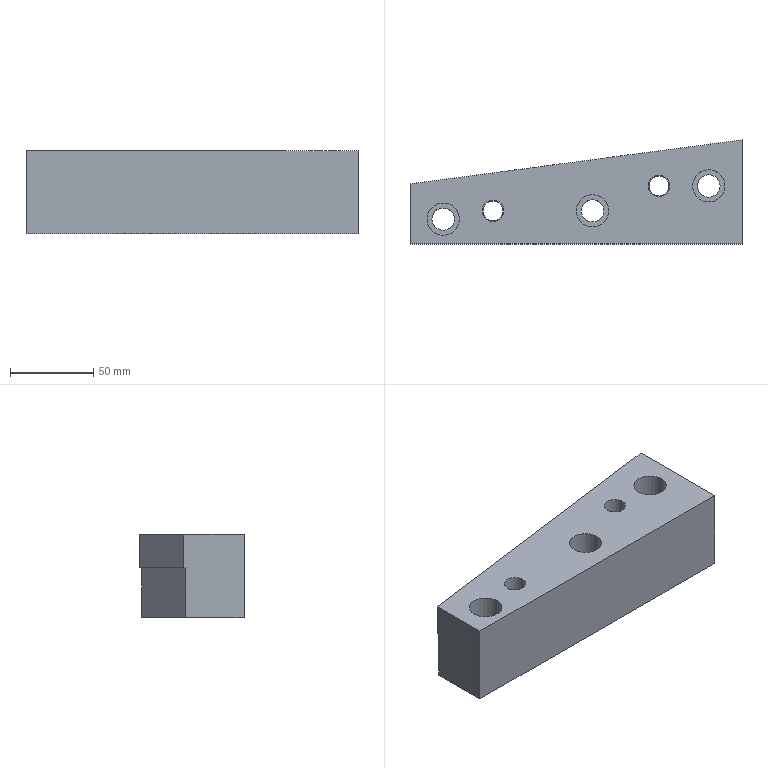Part | NX | features solid 2 | 1 solid | 23 faces | box 200 x 62.717 x 50 mm | volume 447168 mm3 | plane 11 | cylinder 10 | spline 2 | commonest cylinder face diameters 13.5 x3 19.5 x3 12 x2 13 x2
STEP:
#1=CARTESIAN_POINT('',(251.,105.,-50.));
#2=VERTEX_POINT('',#1);
#3=CARTESIAN_POINT('',(245.,105.,-50.));
#4=DIRECTION('',(0.,0.,1.));
#5=DIRECTION('',(1.,0.,0.));
#6=AXIS2_PLACEMENT_3D('',#3,#4,#5);
#7=CIRCLE('',#6,6.);
#8=EDGE_CURVE('',#2,#2,#7,.T.);
#9=ORIENTED_EDGE('',*,*,#8,.T.);
#10=EDGE_LOOP('',(#9));
#11=FACE_BOUND('',#10,.T.);
#12=CARTESIAN_POINT('',(151.,90.,-50.));
#13=VERTEX_POINT('',#12);
#14=CARTESIAN_POINT('',(145.,90.,-50.));
#15=DIRECTION('',(0.,0.,1.));
#16=DIRECTION('',(1.,0.,0.));
#17=AXIS2_PLACEMENT_3D('',#14,#15,#16);
#18=CIRCLE('',#17,6.);
#19=EDGE_CURVE('',#13,#13,#18,.T.);
#20=ORIENTED_EDGE('',*,*,#19,.T.);
#21=EDGE_LOOP('',(#20));
#22=FACE_BOUND('',#21,.T.);
#23=CARTESIAN_POINT('',(211.75,90.,-50.));
#24=VERTEX_POINT('',#23);
#25=CARTESIAN_POINT('',(205.,90.,-50.));
#26=DIRECTION('',(0.,0.,1.));
#27=DIRECTION('',(1.,0.,0.));
#28=AXIS2_PLACEMENT_3D('',#25,#26,#27);
#29=CIRCLE('',#28,6.75);
#30=EDGE_CURVE('',#24,#24,#29,.T.);
#31=ORIENTED_EDGE('',*,*,#30,.T.);
#32=EDGE_LOOP('',(#31));
#33=FACE_BOUND('',#32,.T.);
#34=CARTESIAN_POINT('',(281.75,105.,-50.));
#35=VERTEX_POINT('',#34);
#36=CARTESIAN_POINT('',(275.,105.,-50.));
#37=DIRECTION('',(0.,0.,1.));
#38=DIRECTION('',(1.,0.,0.));
#39=AXIS2_PLACEMENT_3D('',#36,#37,#38);
#40=CIRCLE('',#39,6.75);
#41=EDGE_CURVE('',#35,#35,#40,.T.);
#42=ORIENTED_EDGE('',*,*,#41,.T.);
#43=EDGE_LOOP('',(#42));
#44=FACE_BOUND('',#43,.T.);
#45=CARTESIAN_POINT('',(121.75,85.,-50.));
#46=VERTEX_POINT('',#45);
#47=CARTESIAN_POINT('',(115.,85.,-50.));
#48=DIRECTION('',(0.,0.,1.));
#49=DIRECTION('',(1.,0.,0.));
#50=AXIS2_PLACEMENT_3D('',#47,#48,#49);
#51=CIRCLE('',#50,6.75);
#52=EDGE_CURVE('',#46,#46,#51,.T.);
#53=ORIENTED_EDGE('',*,*,#52,.T.);
#54=EDGE_LOOP('',(#53));
#55=FACE_BOUND('',#54,.T.);
#56=CARTESIAN_POINT('',(95.,70.,-50.));
#57=VERTEX_POINT('',#56);
#58=CARTESIAN_POINT('',(95.,105.2,-50.));
#59=VERTEX_POINT('',#58);
#60=CARTESIAN_POINT('',(95.,35.09,-50.));
#61=DIRECTION('',(0.,1.,0.));
#62=VECTOR('',#61,1000.);
#63=LINE('',#60,#62);
#64=EDGE_CURVE('',#57,#59,#63,.T.);
#65=ORIENTED_EDGE('',*,*,#64,.T.);
#66=CARTESIAN_POINT('',(295.,131.707,-50.));
#67=VERTEX_POINT('',#66);
#68=CARTESIAN_POINT('',(95.,105.2,-50.));
#69=CARTESIAN_POINT('',(128.341,109.558,-50.));
#70=CARTESIAN_POINT('',(178.34,116.191,-50.));
#71=CARTESIAN_POINT('',(245.019,124.939,-50.));
#72=CARTESIAN_POINT('',(278.357,129.318,-50.));
#73=CARTESIAN_POINT('',(295.,131.707,-50.));
#74=B_SPLINE_CURVE_WITH_KNOTS('',3,(#68,#69,#70,#71,#72,#73),.UNSPECIFIED.,.F.,.F.,(4,1,1,4),(0.,0.1009,0.1513,0.2017),.UNSPECIFIED.);
#75=EDGE_CURVE('',#59,#67,#74,.T.);
#76=ORIENTED_EDGE('',*,*,#75,.T.);
#77=CARTESIAN_POINT('',(295.,70.,-50.));
#78=VERTEX_POINT('',#77);
#79=CARTESIAN_POINT('',(295.,35.09,-50.));
#80=DIRECTION('',(0.,-1.,0.));
#81=VECTOR('',#80,1000.);
#82=LINE('',#79,#81);
#83=EDGE_CURVE('',#67,#78,#82,.T.);
#84=ORIENTED_EDGE('',*,*,#83,.T.);
#85=CARTESIAN_POINT('',(-415.478,70.,-50.));
#86=DIRECTION('',(-1.,0.,0.));
#87=VECTOR('',#86,1000.);
#88=LINE('',#85,#87);
#89=EDGE_CURVE('',#78,#57,#88,.T.);
#90=ORIENTED_EDGE('',*,*,#89,.T.);
#91=EDGE_LOOP('',(#65,#76,#84,#90));
#92=FACE_BOUND('',#91,.T.);
#93=CARTESIAN_POINT('',(-415.478,35.09,-50.));
#94=DIRECTION('',(0.,0.,1.));
#95=DIRECTION('',(1.,0.,0.));
#96=AXIS2_PLACEMENT_3D('',#93,#94,#95);
#97=PLANE('',#96);
#98=ADVANCED_FACE('',(#11,#22,#33,#44,#55,#92),#97,.F.);
#99=CARTESIAN_POINT('',(295.,70.,0.));
#100=VERTEX_POINT('',#99);
#101=CARTESIAN_POINT('',(295.,70.,0.));
#102=DIRECTION('',(0.,0.,1.));
#103=VECTOR('',#102,1000.);
#104=LINE('',#101,#103);
#105=EDGE_CURVE('',#78,#100,#104,.T.);
#106=ORIENTED_EDGE('',*,*,#105,.T.);
#107=CARTESIAN_POINT('',(95.,70.,0.));
#108=VERTEX_POINT('',#107);
#109=CARTESIAN_POINT('',(-470.381,70.,0.));
#110=DIRECTION('',(1.,0.,0.));
#111=VECTOR('',#110,1000.);
#112=LINE('',#109,#111);
#113=EDGE_CURVE('',#108,#100,#112,.T.);
#114=ORIENTED_EDGE('',*,*,#113,.F.);
#115=CARTESIAN_POINT('',(95.,70.,0.));
#116=DIRECTION('',(0.,0.,-1.));
#117=VECTOR('',#116,1000.);
#118=LINE('',#115,#117);
#119=EDGE_CURVE('',#108,#57,#118,.T.);
#120=ORIENTED_EDGE('',*,*,#119,.T.);
#121=ORIENTED_EDGE('',*,*,#89,.F.);
#122=EDGE_LOOP('',(#106,#114,#120,#121));
#123=FACE_BOUND('',#122,.T.);
#124=CARTESIAN_POINT('',(180.,70.,0.));
#125=DIRECTION('',(0.,1.,0.));
#126=DIRECTION('',(0.,0.,1.));
#127=AXIS2_PLACEMENT_3D('',#124,#125,#126);
#128=PLANE('',#127);
#129=ADVANCED_FACE('',(#123),#128,.F.);
#130=CARTESIAN_POINT('',(238.5,105.,0.));
#131=VERTEX_POINT('',#130);
#132=CARTESIAN_POINT('',(245.,105.,0.));
#133=DIRECTION('',(0.,0.,-1.));
#134=DIRECTION('',(-1.,0.,0.));
#135=AXIS2_PLACEMENT_3D('',#132,#133,#134);
#136=CIRCLE('',#135,6.5);
#137=EDGE_CURVE('',#131,#131,#136,.T.);
#138=ORIENTED_EDGE('',*,*,#137,.T.);
#139=EDGE_LOOP('',(#138));
#140=FACE_BOUND('',#139,.T.);
#141=CARTESIAN_POINT('',(138.5,90.,0.));
#142=VERTEX_POINT('',#141);
#143=CARTESIAN_POINT('',(145.,90.,0.));
#144=DIRECTION('',(0.,0.,-1.));
#145=DIRECTION('',(-1.,0.,0.));
#146=AXIS2_PLACEMENT_3D('',#143,#144,#145);
#147=CIRCLE('',#146,6.5);
#148=EDGE_CURVE('',#142,#142,#147,.T.);
#149=ORIENTED_EDGE('',*,*,#148,.T.);
#150=EDGE_LOOP('',(#149));
#151=FACE_BOUND('',#150,.T.);
#152=CARTESIAN_POINT('',(195.25,90.,0.));
#153=VERTEX_POINT('',#152);
#154=CARTESIAN_POINT('',(205.,90.,0.));
#155=DIRECTION('',(0.,0.,-1.));
#156=DIRECTION('',(-1.,0.,0.));
#157=AXIS2_PLACEMENT_3D('',#154,#155,#156);
#158=CIRCLE('',#157,9.75);
#159=EDGE_CURVE('',#153,#153,#158,.T.);
#160=ORIENTED_EDGE('',*,*,#159,.T.);
#161=EDGE_LOOP('',(#160));
#162=FACE_BOUND('',#161,.T.);
#163=CARTESIAN_POINT('',(265.25,105.,0.));
#164=VERTEX_POINT('',#163);
#165=CARTESIAN_POINT('',(275.,105.,0.));
#166=DIRECTION('',(0.,0.,-1.));
#167=DIRECTION('',(-1.,0.,0.));
#168=AXIS2_PLACEMENT_3D('',#165,#166,#167);
#169=CIRCLE('',#168,9.75);
#170=EDGE_CURVE('',#164,#164,#169,.T.);
#171=ORIENTED_EDGE('',*,*,#170,.T.);
#172=EDGE_LOOP('',(#171));
#173=FACE_BOUND('',#172,.T.);
#174=CARTESIAN_POINT('',(105.25,85.,0.));
#175=VERTEX_POINT('',#174);
#176=CARTESIAN_POINT('',(115.,85.,0.));
#177=DIRECTION('',(0.,0.,-1.));
#178=DIRECTION('',(-1.,0.,0.));
#179=AXIS2_PLACEMENT_3D('',#176,#177,#178);
#180=CIRCLE('',#179,9.75);
#181=EDGE_CURVE('',#175,#175,#180,.T.);
#182=ORIENTED_EDGE('',*,*,#181,.T.);
#183=EDGE_LOOP('',(#182));
#184=FACE_BOUND('',#183,.T.);
#185=CARTESIAN_POINT('',(295.,132.717,0.));
#186=VERTEX_POINT('',#185);
#187=CARTESIAN_POINT('',(295.,-222.,0.));
#188=DIRECTION('',(0.,1.,0.));
#189=VECTOR('',#188,1000.);
#190=LINE('',#187,#189);
#191=EDGE_CURVE('',#100,#186,#190,.T.);
#192=ORIENTED_EDGE('',*,*,#191,.T.);
#193=CARTESIAN_POINT('',(95.,106.209,0.));
#194=VERTEX_POINT('',#193);
#195=CARTESIAN_POINT('',(95.,106.209,0.));
#196=CARTESIAN_POINT('',(128.341,110.566,0.));
#197=CARTESIAN_POINT('',(178.341,117.199,0.));
#198=CARTESIAN_POINT('',(245.019,125.948,0.));
#199=CARTESIAN_POINT('',(278.357,130.326,0.));
#200=CARTESIAN_POINT('',(295.,132.717,0.));
#201=B_SPLINE_CURVE_WITH_KNOTS('',3,(#195,#196,#197,#198,#199,#200),.UNSPECIFIED.,.F.,.F.,(4,1,1,4),(0.,0.1009,0.1513,0.2017),.UNSPECIFIED.);
#202=EDGE_CURVE('',#194,#186,#201,.T.);
#203=ORIENTED_EDGE('',*,*,#202,.F.);
#204=CARTESIAN_POINT('',(95.,-222.,0.));
#205=DIRECTION('',(0.,-1.,0.));
#206=VECTOR('',#205,1000.);
#207=LINE('',#204,#206);
#208=EDGE_CURVE('',#194,#108,#207,.T.);
#209=ORIENTED_EDGE('',*,*,#208,.T.);
#210=ORIENTED_EDGE('',*,*,#113,.T.);
#211=EDGE_LOOP('',(#192,#203,#209,#210));
#212=FACE_BOUND('',#211,.T.);
#213=CARTESIAN_POINT('',(-470.381,-222.,0.));
#214=DIRECTION('',(0.,0.,-1.));
#215=DIRECTION('',(-1.,0.,0.));
#216=AXIS2_PLACEMENT_3D('',#213,#214,#215);
#217=PLANE('',#216);
#218=ADVANCED_FACE('',(#140,#151,#162,#173,#184,#212),#217,.F.);
#219=CARTESIAN_POINT('',(295.,132.717,-20.));
#220=VERTEX_POINT('',#219);
#221=CARTESIAN_POINT('',(295.,132.717,-10.));
#222=DIRECTION('',(0.,0.,-1.));
#223=VECTOR('',#222,1000.);
#224=LINE('',#221,#223);
#225=EDGE_CURVE('',#186,#220,#224,.T.);
#226=ORIENTED_EDGE('',*,*,#225,.T.);
#227=CARTESIAN_POINT('',(95.,106.209,-20.));
#228=VERTEX_POINT('',#227);
#229=CARTESIAN_POINT('',(-190.231,-121.49,-20.));
#230=CARTESIAN_POINT('',(-188.654,-121.152,-20.));
#231=CARTESIAN_POINT('',(-185.47,-120.627,-20.));
#232=CARTESIAN_POINT('',(-180.656,-120.141,-20.));
#233=CARTESIAN_POINT('',(-175.882,-119.326,-20.));
#234=CARTESIAN_POINT('',(-169.679,-117.528,-20.));
#235=CARTESIAN_POINT('',(-162.185,-114.539,-20.));
#236=CARTESIAN_POINT('',(-153.086,-111.254,-20.));
#237=CARTESIAN_POINT('',(-144.031,-107.845,-20.));
#238=CARTESIAN_POINT('',(-136.465,-105.061,-20.));
#239=CARTESIAN_POINT('',(-130.418,-102.814,-20.));
#240=CARTESIAN_POINT('',(-125.812,-101.329,-20.));
#241=CARTESIAN_POINT('',(-121.306,-99.566,-20.));
#242=CARTESIAN_POINT('',(-116.876,-97.626,-20.));
#243=CARTESIAN_POINT('',(-112.335,-95.923,-20.));
#244=CARTESIAN_POINT('',(-107.564,-95.05,-20.));
#245=CARTESIAN_POINT('',(-102.756,-94.525,-20.));
#246=CARTESIAN_POINT('',(-96.349,-93.771,-20.));
#247=CARTESIAN_POINT('',(-89.902,-93.468,-20.));
#248=CARTESIAN_POINT('',(-83.452,-93.448,-20.));
#249=CARTESIAN_POINT('',(-77.002,-93.469,-20.));
#250=CARTESIAN_POINT('',(-68.939,-93.411,-20.));
#251=CARTESIAN_POINT('',(-56.04,-93.3,-20.));
#252=CARTESIAN_POINT('',(-33.465,-93.184,-20.));
#253=CARTESIAN_POINT('',(-7.666,-93.074,-20.));
#254=CARTESIAN_POINT('',(14.907,-92.653,-20.));
#255=CARTESIAN_POINT('',(27.794,-92.068,-20.));
#256=CARTESIAN_POINT('',(40.668,-91.245,-20.));
#257=CARTESIAN_POINT('',(51.917,-90.291,-20.));
#258=CARTESIAN_POINT('',(61.528,-89.174,-20.));
#259=CARTESIAN_POINT('',(67.939,-88.466,-20.));
#260=CARTESIAN_POINT('',(79.125,-86.95,-20.));
#261=CARTESIAN_POINT('',(95.161,-85.253,-20.));
#262=CARTESIAN_POINT('',(114.404,-83.21,-20.));
#263=CARTESIAN_POINT('',(133.568,-80.524,-20.));
#264=CARTESIAN_POINT('',(152.734,-77.861,-20.));
#265=CARTESIAN_POINT('',(171.916,-75.326,-20.));
#266=CARTESIAN_POINT('',(191.055,-72.413,-20.));
#267=CARTESIAN_POINT('',(207.17,-71.468,-20.));
#268=CARTESIAN_POINT('',(219.951,-69.697,-20.));
#269=CARTESIAN_POINT('',(232.724,-67.899,-20.));
#270=CARTESIAN_POINT('',(248.708,-65.766,-20.));
#271=CARTESIAN_POINT('',(267.87,-63.074,-20.));
#272=CARTESIAN_POINT('',(287.038,-60.44,-20.));
#273=CARTESIAN_POINT('',(301.448,-58.682,-20.));
#274=CARTESIAN_POINT('',(310.976,-56.987,-20.));
#275=CARTESIAN_POINT('',(314.916,-56.135,-20.));
#276=CARTESIAN_POINT('',(318.052,-55.382,-20.));
#277=CARTESIAN_POINT('',(320.39,-54.76,-20.));
#278=CARTESIAN_POINT('',(322.686,-53.981,-20.));
#279=CARTESIAN_POINT('',(325.595,-52.578,-20.));
#280=CARTESIAN_POINT('',(328.769,-50.098,-20.));
#281=CARTESIAN_POINT('',(332.247,-46.69,-20.));
#282=CARTESIAN_POINT('',(335.795,-43.406,-20.));
#283=CARTESIAN_POINT('',(343.661,-37.758,-20.));
#284=CARTESIAN_POINT('',(355.164,-28.914,-20.));
#285=CARTESIAN_POINT('',(370.422,-17.018,-20.));
#286=CARTESIAN_POINT('',(383.264,-7.249,-20.));
#287=CARTESIAN_POINT('',(392.416,-0.6713,-20.));
#288=CARTESIAN_POINT('',(396.953,2.733,-20.));
#289=CARTESIAN_POINT('',(398.886,5.372,-20.));
#290=CARTESIAN_POINT('',(399.725,7.654,-20.));
#291=CARTESIAN_POINT('',(399.76,10.078,-20.));
#292=CARTESIAN_POINT('',(399.483,13.317,-20.));
#293=CARTESIAN_POINT('',(399.712,17.34,-20.));
#294=CARTESIAN_POINT('',(399.612,22.179,-20.));
#295=CARTESIAN_POINT('',(399.633,31.854,-20.));
#296=CARTESIAN_POINT('',(399.593,46.366,-20.));
#297=CARTESIAN_POINT('',(399.637,62.491,-20.));
#298=CARTESIAN_POINT('',(399.588,73.779,-20.));
#299=CARTESIAN_POINT('',(399.652,79.422,-20.));
#300=CARTESIAN_POINT('',(399.59,82.647,-20.));
#301=CARTESIAN_POINT('',(399.564,85.065,-20.));
#302=CARTESIAN_POINT('',(399.725,87.486,-20.));
#303=CARTESIAN_POINT('',(399.756,89.902,-20.));
#304=CARTESIAN_POINT('',(399.247,92.301,-20.));
#305=CARTESIAN_POINT('',(397.362,95.008,-20.));
#306=CARTESIAN_POINT('',(393.635,96.774,-20.));
#307=CARTESIAN_POINT('',(389.279,98.826,-20.));
#308=CARTESIAN_POINT('',(384.732,100.498,-20.));
#309=CARTESIAN_POINT('',(378.765,102.95,-20.));
#310=CARTESIAN_POINT('',(362.589,110.229,-20.));
#311=CARTESIAN_POINT('',(344.928,118.135,-20.));
#312=CARTESIAN_POINT('',(327.281,126.072,-20.));
#313=CARTESIAN_POINT('',(319.932,129.381,-20.));
#314=CARTESIAN_POINT('',(314.075,132.102,-20.));
#315=CARTESIAN_POINT('',(309.387,133.376,-20.));
#316=CARTESIAN_POINT('',(304.547,133.785,-20.));
#317=CARTESIAN_POINT('',(299.716,133.401,-20.));
#318=CARTESIAN_POINT('',(294.929,132.704,-20.));
#319=CARTESIAN_POINT('',(288.543,131.8,-20.));
#320=CARTESIAN_POINT('',(277.364,130.241,-20.));
#321=CARTESIAN_POINT('',(242.2,125.552,-20.));
#322=CARTESIAN_POINT('',(184.637,118.048,-20.));
#323=CARTESIAN_POINT('',(120.701,109.541,-20.));
#324=CARTESIAN_POINT('',(69.531,102.902,-20.));
#325=CARTESIAN_POINT('',(40.777,98.94,-20.));
#326=CARTESIAN_POINT('',(21.566,96.615,-20.));
#327=CARTESIAN_POINT('',(8.743,95.212,-20.));
#328=CARTESIAN_POINT('',(-7.301,93.575,-20.));
#329=CARTESIAN_POINT('',(-26.625,92.505,-20.));
#330=CARTESIAN_POINT('',(-45.971,92.017,-20.));
#331=CARTESIAN_POINT('',(-62.09,91.675,-20.));
#332=CARTESIAN_POINT('',(-74.987,91.256,-20.));
#333=CARTESIAN_POINT('',(-84.664,91.165,-20.));
#334=CARTESIAN_POINT('',(-94.319,91.781,-20.));
#335=CARTESIAN_POINT('',(-103.929,92.966,-20.));
#336=CARTESIAN_POINT('',(-113.495,94.403,-20.));
#337=CARTESIAN_POINT('',(-119.856,95.492,-20.));
#338=CARTESIAN_POINT('',(-122.997,96.222,-20.));
#339=B_SPLINE_CURVE_WITH_KNOTS('',3,(#229,#230,#231,#232,#233,#234,#235,#236,#237,#238,#239,#240,#241,#242,#243,#244,#245,#246,#247,#248,#249,#250,#251,#252,#253,#254,#255,#256,#257,#258,#259,#260,#261,#262,#263,#264,#265,#266,#267,#268,#269,#270,#271,#272,#273,#274,#275,#276,#277,#278,#279,#280,#281,#282,#283,#284,#285,#286,#287,#288,#289,#290,#291,#292,#293,#294,#295,#296,#297,#298,#299,#300,#301,#302,#303,#304,#305,#306,#307,#308,#309,#310,#311,#312,#313,#314,#315,#316,#317,#318,#319,#320,#321,#322,#323,#324,#325,#326,#327,#328,#329,#330,#331,#332,#333,#334,#335,#336,#337,#338),.UNSPECIFIED.,.F.,.F.,(4,1,1,1,1,1,1,1,1,1,1,1,1,1,1,1,1,1,1,1,1,1,1,1,1,1,1,1,1,1,1,1,1,1,1,1,1,1,1,1,1,1,1,1,1,1,1,1,1,1,1,1,1,1,1,1,1,1,1,1,1,1,1,1,1,1,1,1,1,1,1,1,1,1,1,1,1,1,1,1,1,1,1,1,1,1,1,1,1,1,1,1,1,1,1,1,1,1,1,1,1,1,1,1,1,1,1,4),(0.4704,0.4724,0.4745,0.4766,0.4786,0.4828,0.4869,0.491,0.4952,0.4972,0.4993,0.5014,0.5035,0.5055,0.5076,0.5097,0.5117,0.5159,0.5179,0.52,0.5241,0.5283,0.5366,0.5531,0.5614,0.5655,0.5697,0.5779,0.58,0.5821,0.5862,0.5945,0.6028,0.611,0.6193,0.6276,0.6359,0.6441,0.6483,0.6524,0.6607,0.669,0.6772,0.6855,0.6876,0.6897,0.6907,0.6917,0.6928,0.6938,0.6959,0.6979,0.7,0.7021,0.7103,0.7186,0.7269,0.731,0.7331,0.7341,0.7352,0.7362,0.7372,0.7393,0.7414,0.7435,0.7517,0.76,0.7641,0.7662,0.7672,0.7683,0.7693,0.7703,0.7714,0.7724,0.7745,0.7766,0.7786,0.7807,0.7848,0.8014,0.8055,0.8097,0.8117,0.8138,0.8159,0.8179,0.82,0.8221,0.8262,0.8345,0.8676,0.9007,0.9172,0.9338,0.9379,0.9421,0.9503,0.9586,0.9669,0.9752,0.9793,0.9834,0.9876,0.9917,0.9959,1.),.UNSPECIFIED.);
#340=EDGE_CURVE('',#220,#228,#339,.T.);
#341=ORIENTED_EDGE('',*,*,#340,.T.);
#342=CARTESIAN_POINT('',(95.,106.209,-10.));
#343=DIRECTION('',(0.,0.,-1.));
#344=VECTOR('',#343,1000.);
#345=LINE('',#342,#344);
#346=EDGE_CURVE('',#228,#194,#345,.F.);
#347=ORIENTED_EDGE('',*,*,#346,.T.);
#348=ORIENTED_EDGE('',*,*,#202,.T.);
#349=EDGE_LOOP('',(#226,#341,#347,#348));
#350=FACE_BOUND('',#349,.T.);
#351=CARTESIAN_POINT('',(295.,132.717,0.));
#352=CARTESIAN_POINT('',(295.,132.717,-20.));
#353=CARTESIAN_POINT('',(278.359,130.327,0.));
#354=CARTESIAN_POINT('',(278.359,130.327,-20.));
#355=CARTESIAN_POINT('',(245.019,125.948,0.));
#356=CARTESIAN_POINT('',(245.019,125.948,-20.));
#357=CARTESIAN_POINT('',(178.341,117.199,0.));
#358=CARTESIAN_POINT('',(178.341,117.199,-20.));
#359=CARTESIAN_POINT('',(128.341,110.566,0.));
#360=CARTESIAN_POINT('',(128.341,110.566,-20.));
#361=CARTESIAN_POINT('',(95.,106.209,0.));
#362=CARTESIAN_POINT('',(95.,106.209,-20.));
#363=B_SPLINE_SURFACE_WITH_KNOTS('',3,1,((#351,#352),(#353,#354),(#355,#356),(#357,#358),(#359,#360),(#361,#362)),.SURF_OF_LINEAR_EXTRUSION.,.F.,.F.,.F.,(4,1,1,4),(2,2),(0.82,0.8415,0.8631,0.9063),(0.,1.),.UNSPECIFIED.);
#364=ADVANCED_FACE('',(#350),#363,.F.);
#365=CARTESIAN_POINT('',(295.,131.707,-20.));
#366=VERTEX_POINT('',#365);
#367=CARTESIAN_POINT('',(295.,131.707,-60.));
#368=DIRECTION('',(0.,0.,-1.));
#369=VECTOR('',#368,1000.);
#370=LINE('',#367,#369);
#371=EDGE_CURVE('',#67,#366,#370,.F.);
#372=ORIENTED_EDGE('',*,*,#371,.T.);
#373=CARTESIAN_POINT('',(295.,32.206,-20.));
#374=DIRECTION('',(0.,1.,0.));
#375=VECTOR('',#374,1000.);
#376=LINE('',#373,#375);
#377=EDGE_CURVE('',#366,#220,#376,.T.);
#378=ORIENTED_EDGE('',*,*,#377,.T.);
#379=ORIENTED_EDGE('',*,*,#225,.F.);
#380=ORIENTED_EDGE('',*,*,#191,.F.);
#381=ORIENTED_EDGE('',*,*,#105,.F.);
#382=ORIENTED_EDGE('',*,*,#83,.F.);
#383=EDGE_LOOP('',(#372,#378,#379,#380,#381,#382));
#384=FACE_BOUND('',#383,.T.);
#385=CARTESIAN_POINT('',(295.,32.206,-25.));
#386=DIRECTION('',(-1.,0.,0.));
#387=DIRECTION('',(0.,0.,1.));
#388=AXIS2_PLACEMENT_3D('',#385,#386,#387);
#389=PLANE('',#388);
#390=ADVANCED_FACE('',(#384),#389,.F.);
#391=ORIENTED_EDGE('',*,*,#346,.F.);
#392=CARTESIAN_POINT('',(95.,105.2,-20.));
#393=VERTEX_POINT('',#392);
#394=CARTESIAN_POINT('',(95.,83.097,-20.));
#395=DIRECTION('',(0.,-1.,0.));
#396=VECTOR('',#395,1000.);
#397=LINE('',#394,#396);
#398=EDGE_CURVE('',#228,#393,#397,.T.);
#399=ORIENTED_EDGE('',*,*,#398,.T.);
#400=CARTESIAN_POINT('',(95.,105.2,-60.));
#401=DIRECTION('',(0.,0.,-1.));
#402=VECTOR('',#401,1000.);
#403=LINE('',#400,#402);
#404=EDGE_CURVE('',#393,#59,#403,.T.);
#405=ORIENTED_EDGE('',*,*,#404,.T.);
#406=ORIENTED_EDGE('',*,*,#64,.F.);
#407=ORIENTED_EDGE('',*,*,#119,.F.);
#408=ORIENTED_EDGE('',*,*,#208,.F.);
#409=EDGE_LOOP('',(#391,#399,#405,#406,#407,#408));
#410=FACE_BOUND('',#409,.T.);
#411=CARTESIAN_POINT('',(95.,83.097,-25.));
#412=DIRECTION('',(1.,0.,0.));
#413=DIRECTION('',(0.,0.,-1.));
#414=AXIS2_PLACEMENT_3D('',#411,#412,#413);
#415=PLANE('',#414);
#416=ADVANCED_FACE('',(#410),#415,.F.);
#417=CARTESIAN_POINT('',(108.25,85.,-15.));
#418=VERTEX_POINT('',#417);
#419=CARTESIAN_POINT('',(115.,85.,-15.));
#420=DIRECTION('',(0.,0.,-1.));
#421=DIRECTION('',(-1.,0.,0.));
#422=AXIS2_PLACEMENT_3D('',#419,#420,#421);
#423=CIRCLE('',#422,6.75);
#424=EDGE_CURVE('',#418,#418,#423,.T.);
#425=ORIENTED_EDGE('',*,*,#424,.F.);
#426=EDGE_LOOP('',(#425));
#427=FACE_BOUND('',#426,.T.);
#428=ORIENTED_EDGE('',*,*,#52,.F.);
#429=EDGE_LOOP('',(#428));
#430=FACE_BOUND('',#429,.T.);
#431=CARTESIAN_POINT('',(115.,85.,-100.));
#432=DIRECTION('',(0.,0.,-1.));
#433=DIRECTION('',(-1.,0.,0.));
#434=AXIS2_PLACEMENT_3D('',#431,#432,#433);
#435=CYLINDRICAL_SURFACE('',#434,6.75);
#436=ADVANCED_FACE('',(#427,#430),#435,.F.);
#437=ORIENTED_EDGE('',*,*,#424,.T.);
#438=EDGE_LOOP('',(#437));
#439=FACE_BOUND('',#438,.T.);
#440=CARTESIAN_POINT('',(105.25,85.,-15.));
#441=VERTEX_POINT('',#440);
#442=CARTESIAN_POINT('',(115.,85.,-15.));
#443=DIRECTION('',(0.,0.,-1.));
#444=DIRECTION('',(-1.,0.,0.));
#445=AXIS2_PLACEMENT_3D('',#442,#443,#444);
#446=CIRCLE('',#445,9.75);
#447=EDGE_CURVE('',#441,#441,#446,.T.);
#448=ORIENTED_EDGE('',*,*,#447,.F.);
#449=EDGE_LOOP('',(#448));
#450=FACE_BOUND('',#449,.T.);
#451=CARTESIAN_POINT('',(115.,90.,-15.));
#452=DIRECTION('',(0.,0.,-1.));
#453=DIRECTION('',(-1.,0.,0.));
#454=AXIS2_PLACEMENT_3D('',#451,#452,#453);
#455=PLANE('',#454);
#456=ADVANCED_FACE('',(#439,#450),#455,.F.);
#457=ORIENTED_EDGE('',*,*,#447,.T.);
#458=EDGE_LOOP('',(#457));
#459=FACE_BOUND('',#458,.T.);
#460=ORIENTED_EDGE('',*,*,#181,.F.);
#461=EDGE_LOOP('',(#460));
#462=FACE_BOUND('',#461,.T.);
#463=CARTESIAN_POINT('',(115.,85.,0.));
#464=DIRECTION('',(0.,0.,-1.));
#465=DIRECTION('',(-1.,0.,0.));
#466=AXIS2_PLACEMENT_3D('',#463,#464,#465);
#467=CYLINDRICAL_SURFACE('',#466,9.75);
#468=ADVANCED_FACE('',(#459,#462),#467,.F.);
#469=CARTESIAN_POINT('',(268.25,105.,-15.));
#470=VERTEX_POINT('',#469);
#471=CARTESIAN_POINT('',(275.,105.,-15.));
#472=DIRECTION('',(0.,0.,-1.));
#473=DIRECTION('',(-1.,0.,0.));
#474=AXIS2_PLACEMENT_3D('',#471,#472,#473);
#475=CIRCLE('',#474,6.75);
#476=EDGE_CURVE('',#470,#470,#475,.T.);
#477=ORIENTED_EDGE('',*,*,#476,.F.);
#478=EDGE_LOOP('',(#477));
#479=FACE_BOUND('',#478,.T.);
#480=ORIENTED_EDGE('',*,*,#41,.F.);
#481=EDGE_LOOP('',(#480));
#482=FACE_BOUND('',#481,.T.);
#483=CARTESIAN_POINT('',(275.,105.,-100.));
#484=DIRECTION('',(0.,0.,-1.));
#485=DIRECTION('',(-1.,0.,0.));
#486=AXIS2_PLACEMENT_3D('',#483,#484,#485);
#487=CYLINDRICAL_SURFACE('',#486,6.75);
#488=ADVANCED_FACE('',(#479,#482),#487,.F.);
#489=ORIENTED_EDGE('',*,*,#476,.T.);
#490=EDGE_LOOP('',(#489));
#491=FACE_BOUND('',#490,.T.);
#492=CARTESIAN_POINT('',(265.25,105.,-15.));
#493=VERTEX_POINT('',#492);
#494=CARTESIAN_POINT('',(275.,105.,-15.));
#495=DIRECTION('',(0.,0.,-1.));
#496=DIRECTION('',(-1.,0.,0.));
#497=AXIS2_PLACEMENT_3D('',#494,#495,#496);
#498=CIRCLE('',#497,9.75);
#499=EDGE_CURVE('',#493,#493,#498,.T.);
#500=ORIENTED_EDGE('',*,*,#499,.F.);
#501=EDGE_LOOP('',(#500));
#502=FACE_BOUND('',#501,.T.);
#503=CARTESIAN_POINT('',(275.,105.,-15.));
#504=DIRECTION('',(0.,0.,-1.));
#505=DIRECTION('',(-1.,0.,0.));
#506=AXIS2_PLACEMENT_3D('',#503,#504,#505);
#507=PLANE('',#506);
#508=ADVANCED_FACE('',(#491,#502),#507,.F.);
#509=ORIENTED_EDGE('',*,*,#499,.T.);
#510=EDGE_LOOP('',(#509));
#511=FACE_BOUND('',#510,.T.);
#512=ORIENTED_EDGE('',*,*,#170,.F.);
#513=EDGE_LOOP('',(#512));
#514=FACE_BOUND('',#513,.T.);
#515=CARTESIAN_POINT('',(275.,105.,0.));
#516=DIRECTION('',(0.,0.,-1.));
#517=DIRECTION('',(-1.,0.,0.));
#518=AXIS2_PLACEMENT_3D('',#515,#516,#517);
#519=CYLINDRICAL_SURFACE('',#518,9.75);
#520=ADVANCED_FACE('',(#511,#514),#519,.F.);
#521=CARTESIAN_POINT('',(198.25,90.,-15.));
#522=VERTEX_POINT('',#521);
#523=CARTESIAN_POINT('',(205.,90.,-15.));
#524=DIRECTION('',(0.,0.,-1.));
#525=DIRECTION('',(-1.,0.,0.));
#526=AXIS2_PLACEMENT_3D('',#523,#524,#525);
#527=CIRCLE('',#526,6.75);
#528=EDGE_CURVE('',#522,#522,#527,.T.);
#529=ORIENTED_EDGE('',*,*,#528,.F.);
#530=EDGE_LOOP('',(#529));
#531=FACE_BOUND('',#530,.T.);
#532=ORIENTED_EDGE('',*,*,#30,.F.);
#533=EDGE_LOOP('',(#532));
#534=FACE_BOUND('',#533,.T.);
#535=CARTESIAN_POINT('',(205.,90.,-100.));
#536=DIRECTION('',(0.,0.,-1.));
#537=DIRECTION('',(-1.,0.,0.));
#538=AXIS2_PLACEMENT_3D('',#535,#536,#537);
#539=CYLINDRICAL_SURFACE('',#538,6.75);
#540=ADVANCED_FACE('',(#531,#534),#539,.F.);
#541=ORIENTED_EDGE('',*,*,#528,.T.);
#542=EDGE_LOOP('',(#541));
#543=FACE_BOUND('',#542,.T.);
#544=CARTESIAN_POINT('',(195.25,90.,-15.));
#545=VERTEX_POINT('',#544);
#546=CARTESIAN_POINT('',(205.,90.,-15.));
#547=DIRECTION('',(0.,0.,-1.));
#548=DIRECTION('',(-1.,0.,0.));
#549=AXIS2_PLACEMENT_3D('',#546,#547,#548);
#550=CIRCLE('',#549,9.75);
#551=EDGE_CURVE('',#545,#545,#550,.T.);
#552=ORIENTED_EDGE('',*,*,#551,.F.);
#553=EDGE_LOOP('',(#552));
#554=FACE_BOUND('',#553,.T.);
#555=CARTESIAN_POINT('',(205.,90.,-15.));
#556=DIRECTION('',(0.,0.,-1.));
#557=DIRECTION('',(-1.,0.,0.));
#558=AXIS2_PLACEMENT_3D('',#555,#556,#557);
#559=PLANE('',#558);
#560=ADVANCED_FACE('',(#543,#554),#559,.F.);
#561=ORIENTED_EDGE('',*,*,#551,.T.);
#562=EDGE_LOOP('',(#561));
#563=FACE_BOUND('',#562,.T.);
#564=ORIENTED_EDGE('',*,*,#159,.F.);
#565=EDGE_LOOP('',(#564));
#566=FACE_BOUND('',#565,.T.);
#567=CARTESIAN_POINT('',(205.,90.,0.));
#568=DIRECTION('',(0.,0.,-1.));
#569=DIRECTION('',(-1.,0.,0.));
#570=AXIS2_PLACEMENT_3D('',#567,#568,#569);
#571=CYLINDRICAL_SURFACE('',#570,9.75);
#572=ADVANCED_FACE('',(#563,#566),#571,.F.);
#573=CARTESIAN_POINT('',(139.,90.,-20.));
#574=VERTEX_POINT('',#573);
#575=CARTESIAN_POINT('',(145.,90.,-20.));
#576=DIRECTION('',(0.,0.,-1.));
#577=DIRECTION('',(-1.,0.,0.));
#578=AXIS2_PLACEMENT_3D('',#575,#576,#577);
#579=CIRCLE('',#578,6.);
#580=EDGE_CURVE('',#574,#574,#579,.T.);
#581=ORIENTED_EDGE('',*,*,#580,.F.);
#582=EDGE_LOOP('',(#581));
#583=FACE_BOUND('',#582,.T.);
#584=ORIENTED_EDGE('',*,*,#19,.F.);
#585=EDGE_LOOP('',(#584));
#586=FACE_BOUND('',#585,.T.);
#587=CARTESIAN_POINT('',(145.,90.,-100.));
#588=DIRECTION('',(0.,0.,-1.));
#589=DIRECTION('',(-1.,0.,0.));
#590=AXIS2_PLACEMENT_3D('',#587,#588,#589);
#591=CYLINDRICAL_SURFACE('',#590,6.);
#592=ADVANCED_FACE('',(#583,#586),#591,.F.);
#593=ORIENTED_EDGE('',*,*,#580,.T.);
#594=EDGE_LOOP('',(#593));
#595=FACE_BOUND('',#594,.T.);
#596=CARTESIAN_POINT('',(138.5,90.,-20.));
#597=VERTEX_POINT('',#596);
#598=CARTESIAN_POINT('',(145.,90.,-20.));
#599=DIRECTION('',(0.,0.,-1.));
#600=DIRECTION('',(-1.,0.,0.));
#601=AXIS2_PLACEMENT_3D('',#598,#599,#600);
#602=CIRCLE('',#601,6.5);
#603=EDGE_CURVE('',#597,#597,#602,.T.);
#604=ORIENTED_EDGE('',*,*,#603,.F.);
#605=EDGE_LOOP('',(#604));
#606=FACE_BOUND('',#605,.T.);
#607=CARTESIAN_POINT('',(145.,90.,-20.));
#608=DIRECTION('',(0.,0.,-1.));
#609=DIRECTION('',(-1.,0.,0.));
#610=AXIS2_PLACEMENT_3D('',#607,#608,#609);
#611=PLANE('',#610);
#612=ADVANCED_FACE('',(#595,#606),#611,.F.);
#613=ORIENTED_EDGE('',*,*,#603,.T.);
#614=EDGE_LOOP('',(#613));
#615=FACE_BOUND('',#614,.T.);
#616=ORIENTED_EDGE('',*,*,#148,.F.);
#617=EDGE_LOOP('',(#616));
#618=FACE_BOUND('',#617,.T.);
#619=CARTESIAN_POINT('',(145.,90.,0.));
#620=DIRECTION('',(0.,0.,-1.));
#621=DIRECTION('',(-1.,0.,0.));
#622=AXIS2_PLACEMENT_3D('',#619,#620,#621);
#623=CYLINDRICAL_SURFACE('',#622,6.5);
#624=ADVANCED_FACE('',(#615,#618),#623,.F.);
#625=CARTESIAN_POINT('',(239.,105.,-20.));
#626=VERTEX_POINT('',#625);
#627=CARTESIAN_POINT('',(245.,105.,-20.));
#628=DIRECTION('',(0.,0.,-1.));
#629=DIRECTION('',(-1.,0.,0.));
#630=AXIS2_PLACEMENT_3D('',#627,#628,#629);
#631=CIRCLE('',#630,6.);
#632=EDGE_CURVE('',#626,#626,#631,.T.);
#633=ORIENTED_EDGE('',*,*,#632,.F.);
#634=EDGE_LOOP('',(#633));
#635=FACE_BOUND('',#634,.T.);
#636=ORIENTED_EDGE('',*,*,#8,.F.);
#637=EDGE_LOOP('',(#636));
#638=FACE_BOUND('',#637,.T.);
#639=CARTESIAN_POINT('',(245.,105.,-100.));
#640=DIRECTION('',(0.,0.,-1.));
#641=DIRECTION('',(-1.,0.,0.));
#642=AXIS2_PLACEMENT_3D('',#639,#640,#641);
#643=CYLINDRICAL_SURFACE('',#642,6.);
#644=ADVANCED_FACE('',(#635,#638),#643,.F.);
#645=ORIENTED_EDGE('',*,*,#632,.T.);
#646=EDGE_LOOP('',(#645));
#647=FACE_BOUND('',#646,.T.);
#648=CARTESIAN_POINT('',(238.5,105.,-20.));
#649=VERTEX_POINT('',#648);
#650=CARTESIAN_POINT('',(245.,105.,-20.));
#651=DIRECTION('',(0.,0.,-1.));
#652=DIRECTION('',(-1.,0.,0.));
#653=AXIS2_PLACEMENT_3D('',#650,#651,#652);
#654=CIRCLE('',#653,6.5);
#655=EDGE_CURVE('',#649,#649,#654,.T.);
#656=ORIENTED_EDGE('',*,*,#655,.F.);
#657=EDGE_LOOP('',(#656));
#658=FACE_BOUND('',#657,.T.);
#659=CARTESIAN_POINT('',(245.,105.,-20.));
#660=DIRECTION('',(0.,0.,-1.));
#661=DIRECTION('',(-1.,0.,0.));
#662=AXIS2_PLACEMENT_3D('',#659,#660,#661);
#663=PLANE('',#662);
#664=ADVANCED_FACE('',(#647,#658),#663,.F.);
#665=ORIENTED_EDGE('',*,*,#655,.T.);
#666=EDGE_LOOP('',(#665));
#667=FACE_BOUND('',#666,.T.);
#668=ORIENTED_EDGE('',*,*,#137,.F.);
#669=EDGE_LOOP('',(#668));
#670=FACE_BOUND('',#669,.T.);
#671=CARTESIAN_POINT('',(245.,105.,0.));
#672=DIRECTION('',(0.,0.,-1.));
#673=DIRECTION('',(-1.,0.,0.));
#674=AXIS2_PLACEMENT_3D('',#671,#672,#673);
#675=CYLINDRICAL_SURFACE('',#674,6.5);
#676=ADVANCED_FACE('',(#667,#670),#675,.F.);
#677=CARTESIAN_POINT('',(295.,131.707,-20.));
#678=CARTESIAN_POINT('',(278.346,129.316,-20.));
#679=CARTESIAN_POINT('',(245.012,124.938,-20.));
#680=CARTESIAN_POINT('',(178.336,116.19,-20.));
#681=CARTESIAN_POINT('',(128.338,109.557,-20.));
#682=CARTESIAN_POINT('',(95.,105.2,-20.));
#683=B_SPLINE_CURVE_WITH_KNOTS('',3,(#677,#678,#679,#680,#681,#682),.UNSPECIFIED.,.F.,.F.,(4,1,1,4),(0.82,0.8416,0.8632,0.9063),.UNSPECIFIED.);
#684=EDGE_CURVE('',#366,#393,#683,.T.);
#685=ORIENTED_EDGE('',*,*,#684,.T.);
#686=ORIENTED_EDGE('',*,*,#398,.F.);
#687=ORIENTED_EDGE('',*,*,#340,.F.);
#688=ORIENTED_EDGE('',*,*,#377,.F.);
#689=EDGE_LOOP('',(#685,#686,#687,#688));
#690=FACE_BOUND('',#689,.T.);
#691=CARTESIAN_POINT('',(-190.231,-121.49,-20.));
#692=DIRECTION('',(0.,0.,1.));
#693=DIRECTION('',(1.,0.,0.));
#694=AXIS2_PLACEMENT_3D('',#691,#692,#693);
#695=PLANE('',#694);
#696=ADVANCED_FACE('',(#690),#695,.F.);
#697=ORIENTED_EDGE('',*,*,#75,.F.);
#698=ORIENTED_EDGE('',*,*,#404,.F.);
#699=ORIENTED_EDGE('',*,*,#684,.F.);
#700=ORIENTED_EDGE('',*,*,#371,.F.);
#701=EDGE_LOOP('',(#697,#698,#699,#700));
#702=FACE_BOUND('',#701,.T.);
#703=CARTESIAN_POINT('',(295.,131.707,-20.));
#704=CARTESIAN_POINT('',(295.,131.707,-50.));
#705=CARTESIAN_POINT('',(278.346,129.316,-20.));
#706=CARTESIAN_POINT('',(278.346,129.316,-50.));
#707=CARTESIAN_POINT('',(245.012,124.938,-20.));
#708=CARTESIAN_POINT('',(245.012,124.938,-50.));
#709=CARTESIAN_POINT('',(178.336,116.19,-20.));
#710=CARTESIAN_POINT('',(178.336,116.19,-50.));
#711=CARTESIAN_POINT('',(128.338,109.557,-20.));
#712=CARTESIAN_POINT('',(128.338,109.557,-50.));
#713=CARTESIAN_POINT('',(95.,105.2,-20.));
#714=CARTESIAN_POINT('',(95.,105.2,-50.));
#715=B_SPLINE_SURFACE_WITH_KNOTS('',3,1,((#703,#704),(#705,#706),(#707,#708),(#709,#710),(#711,#712),(#713,#714)),.SURF_OF_LINEAR_EXTRUSION.,.F.,.F.,.F.,(4,1,1,4),(2,2),(0.82,0.8416,0.8632,0.9063),(0.,1.),.UNSPECIFIED.);
#716=ADVANCED_FACE('',(#702),#715,.F.);
#717=CLOSED_SHELL('',(#98,#129,#218,#364,#390,#416,#436,#456,#468,#488,#508,#520,#540,#560,#572,#592,#612,#624,#644,#664,#676,#696,#716));
#718=MANIFOLD_SOLID_BREP('',#717);
#719=(LENGTH_UNIT()NAMED_UNIT(*)SI_UNIT(.MILLI.,.METRE.));
#720=UNCERTAINTY_MEASURE_WITH_UNIT(LENGTH_MEASURE(0.0508),#719,'','');
#721=(NAMED_UNIT(*)PLANE_ANGLE_UNIT()SI_UNIT($,.RADIAN.));
#722=(NAMED_UNIT(*)SI_UNIT($,.STERADIAN.)SOLID_ANGLE_UNIT());
#723=(GEOMETRIC_REPRESENTATION_CONTEXT(3)GLOBAL_UNCERTAINTY_ASSIGNED_CONTEXT((#720))GLOBAL_UNIT_ASSIGNED_CONTEXT((#719,#721,#722))REPRESENTATION_CONTEXT('',''));
#724=ADVANCED_BREP_SHAPE_REPRESENTATION('',(#718),#723);